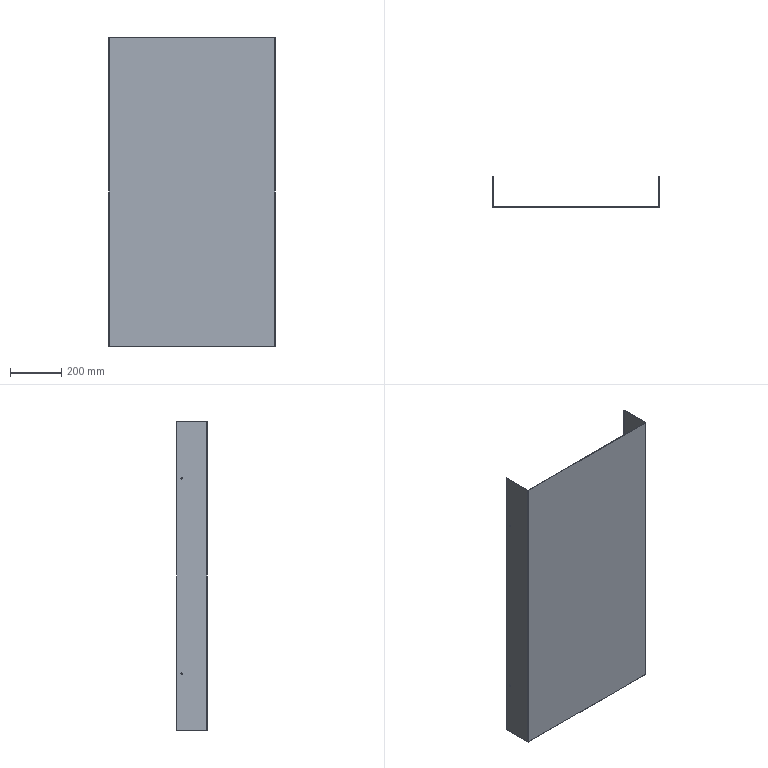Part | SolidWorks | features FlatPattern 1, ICE 1, SMBaseFlange 1, SheetMetal 1 | 1 solid | 30 faces | box 648 x 120 x 1198 mm | volume 2114266 mm3 | plane 18 | cylinder 12 | commonest cylinder face diameters 6 x8 1.473 x2 5.473 x2
STEP:
#1=CARTESIAN_POINT('',(2.,100.,-383.));
#2=VERTEX_POINT('',#1);
#3=CARTESIAN_POINT('',(2.,100.,-377.));
#4=VERTEX_POINT('',#3);
#5=CARTESIAN_POINT('',(2.,100.,-380.));
#6=DIRECTION('',(-1.,0.,0.));
#7=DIRECTION('',(0.,0.,1.));
#8=AXIS2_PLACEMENT_3D('',#5,#6,#7);
#9=CIRCLE('',#8,3.);
#10=EDGE_CURVE('',#2,#4,#9,.T.);
#11=ORIENTED_EDGE('',*,*,#10,.F.);
#12=CARTESIAN_POINT('',(0.,100.,-383.));
#13=VERTEX_POINT('',#12);
#14=CARTESIAN_POINT('',(648.,100.,-383.));
#15=DIRECTION('',(-1.,0.,0.));
#16=VECTOR('',#15,1000.);
#17=LINE('',#14,#16);
#18=EDGE_CURVE('',#2,#13,#17,.T.);
#19=ORIENTED_EDGE('',*,*,#18,.T.);
#20=CARTESIAN_POINT('',(0.,100.,-377.));
#21=VERTEX_POINT('',#20);
#22=CARTESIAN_POINT('',(0.,100.,-380.));
#23=DIRECTION('',(-1.,0.,0.));
#24=DIRECTION('',(0.,0.,1.));
#25=AXIS2_PLACEMENT_3D('',#22,#23,#24);
#26=CIRCLE('',#25,3.);
#27=EDGE_CURVE('',#13,#21,#26,.T.);
#28=ORIENTED_EDGE('',*,*,#27,.T.);
#29=CARTESIAN_POINT('',(648.,100.,-377.));
#30=DIRECTION('',(-1.,0.,0.));
#31=VECTOR('',#30,1000.);
#32=LINE('',#29,#31);
#33=EDGE_CURVE('',#4,#21,#32,.T.);
#34=ORIENTED_EDGE('',*,*,#33,.F.);
#35=EDGE_LOOP('',(#11,#19,#28,#34));
#36=FACE_OUTER_BOUND('',#35,.T.);
#37=CARTESIAN_POINT('',(648.,100.,-380.));
#38=DIRECTION('',(-1.,0.,0.));
#39=DIRECTION('',(0.,0.,1.));
#40=AXIS2_PLACEMENT_3D('',#37,#38,#39);
#41=CYLINDRICAL_SURFACE('',#40,3.);
#42=ADVANCED_FACE('',(#36),#41,.F.);
#43=CARTESIAN_POINT('',(2.,100.,377.));
#44=VERTEX_POINT('',#43);
#45=CARTESIAN_POINT('',(2.,100.,383.));
#46=VERTEX_POINT('',#45);
#47=CARTESIAN_POINT('',(2.,100.,380.));
#48=DIRECTION('',(-1.,0.,0.));
#49=DIRECTION('',(0.,0.,1.));
#50=AXIS2_PLACEMENT_3D('',#47,#48,#49);
#51=CIRCLE('',#50,3.);
#52=EDGE_CURVE('',#44,#46,#51,.T.);
#53=ORIENTED_EDGE('',*,*,#52,.F.);
#54=CARTESIAN_POINT('',(0.,100.,377.));
#55=VERTEX_POINT('',#54);
#56=CARTESIAN_POINT('',(648.,100.,377.));
#57=DIRECTION('',(-1.,0.,0.));
#58=VECTOR('',#57,1000.);
#59=LINE('',#56,#58);
#60=EDGE_CURVE('',#44,#55,#59,.T.);
#61=ORIENTED_EDGE('',*,*,#60,.T.);
#62=CARTESIAN_POINT('',(0.,100.,383.));
#63=VERTEX_POINT('',#62);
#64=CARTESIAN_POINT('',(0.,100.,380.));
#65=DIRECTION('',(-1.,0.,0.));
#66=DIRECTION('',(0.,0.,1.));
#67=AXIS2_PLACEMENT_3D('',#64,#65,#66);
#68=CIRCLE('',#67,3.);
#69=EDGE_CURVE('',#55,#63,#68,.T.);
#70=ORIENTED_EDGE('',*,*,#69,.T.);
#71=CARTESIAN_POINT('',(648.,100.,383.));
#72=DIRECTION('',(-1.,0.,0.));
#73=VECTOR('',#72,1000.);
#74=LINE('',#71,#73);
#75=EDGE_CURVE('',#46,#63,#74,.T.);
#76=ORIENTED_EDGE('',*,*,#75,.F.);
#77=EDGE_LOOP('',(#53,#61,#70,#76));
#78=FACE_OUTER_BOUND('',#77,.T.);
#79=CARTESIAN_POINT('',(648.,100.,380.));
#80=DIRECTION('',(-1.,0.,0.));
#81=DIRECTION('',(0.,0.,1.));
#82=AXIS2_PLACEMENT_3D('',#79,#80,#81);
#83=CYLINDRICAL_SURFACE('',#82,3.);
#84=ADVANCED_FACE('',(#78),#83,.F.);
#85=CARTESIAN_POINT('',(648.,100.,-383.));
#86=VERTEX_POINT('',#85);
#87=CARTESIAN_POINT('',(648.,100.,-377.));
#88=VERTEX_POINT('',#87);
#89=CARTESIAN_POINT('',(648.,100.,-380.));
#90=DIRECTION('',(-1.,0.,0.));
#91=DIRECTION('',(0.,0.,1.));
#92=AXIS2_PLACEMENT_3D('',#89,#90,#91);
#93=CIRCLE('',#92,3.);
#94=EDGE_CURVE('',#86,#88,#93,.T.);
#95=ORIENTED_EDGE('',*,*,#94,.F.);
#96=CARTESIAN_POINT('',(646.,100.,-383.));
#97=VERTEX_POINT('',#96);
#98=CARTESIAN_POINT('',(648.,100.,-383.));
#99=DIRECTION('',(-1.,0.,0.));
#100=VECTOR('',#99,1000.);
#101=LINE('',#98,#100);
#102=EDGE_CURVE('',#86,#97,#101,.T.);
#103=ORIENTED_EDGE('',*,*,#102,.T.);
#104=CARTESIAN_POINT('',(646.,100.,-377.));
#105=VERTEX_POINT('',#104);
#106=CARTESIAN_POINT('',(646.,100.,-380.));
#107=DIRECTION('',(1.,0.,0.));
#108=DIRECTION('',(0.,0.,-1.));
#109=AXIS2_PLACEMENT_3D('',#106,#107,#108);
#110=CIRCLE('',#109,3.);
#111=EDGE_CURVE('',#105,#97,#110,.T.);
#112=ORIENTED_EDGE('',*,*,#111,.F.);
#113=CARTESIAN_POINT('',(648.,100.,-377.));
#114=DIRECTION('',(-1.,0.,0.));
#115=VECTOR('',#114,1000.);
#116=LINE('',#113,#115);
#117=EDGE_CURVE('',#88,#105,#116,.T.);
#118=ORIENTED_EDGE('',*,*,#117,.F.);
#119=EDGE_LOOP('',(#95,#103,#112,#118));
#120=FACE_OUTER_BOUND('',#119,.T.);
#121=CARTESIAN_POINT('',(648.,100.,-380.));
#122=DIRECTION('',(-1.,0.,0.));
#123=DIRECTION('',(0.,0.,1.));
#124=AXIS2_PLACEMENT_3D('',#121,#122,#123);
#125=CYLINDRICAL_SURFACE('',#124,3.);
#126=ADVANCED_FACE('',(#120),#125,.F.);
#127=CARTESIAN_POINT('',(648.,100.,377.));
#128=VERTEX_POINT('',#127);
#129=CARTESIAN_POINT('',(648.,100.,383.));
#130=VERTEX_POINT('',#129);
#131=CARTESIAN_POINT('',(648.,100.,380.));
#132=DIRECTION('',(-1.,0.,0.));
#133=DIRECTION('',(0.,0.,1.));
#134=AXIS2_PLACEMENT_3D('',#131,#132,#133);
#135=CIRCLE('',#134,3.);
#136=EDGE_CURVE('',#128,#130,#135,.T.);
#137=ORIENTED_EDGE('',*,*,#136,.F.);
#138=CARTESIAN_POINT('',(646.,100.,377.));
#139=VERTEX_POINT('',#138);
#140=CARTESIAN_POINT('',(648.,100.,377.));
#141=DIRECTION('',(-1.,0.,0.));
#142=VECTOR('',#141,1000.);
#143=LINE('',#140,#142);
#144=EDGE_CURVE('',#128,#139,#143,.T.);
#145=ORIENTED_EDGE('',*,*,#144,.T.);
#146=CARTESIAN_POINT('',(646.,100.,383.));
#147=VERTEX_POINT('',#146);
#148=CARTESIAN_POINT('',(646.,100.,380.));
#149=DIRECTION('',(1.,0.,0.));
#150=DIRECTION('',(0.,0.,-1.));
#151=AXIS2_PLACEMENT_3D('',#148,#149,#150);
#152=CIRCLE('',#151,3.);
#153=EDGE_CURVE('',#147,#139,#152,.T.);
#154=ORIENTED_EDGE('',*,*,#153,.F.);
#155=CARTESIAN_POINT('',(648.,100.,383.));
#156=DIRECTION('',(-1.,0.,0.));
#157=VECTOR('',#156,1000.);
#158=LINE('',#155,#157);
#159=EDGE_CURVE('',#130,#147,#158,.T.);
#160=ORIENTED_EDGE('',*,*,#159,.F.);
#161=EDGE_LOOP('',(#137,#145,#154,#160));
#162=FACE_OUTER_BOUND('',#161,.T.);
#163=CARTESIAN_POINT('',(648.,100.,380.));
#164=DIRECTION('',(-1.,0.,0.));
#165=DIRECTION('',(0.,0.,1.));
#166=AXIS2_PLACEMENT_3D('',#163,#164,#165);
#167=CYLINDRICAL_SURFACE('',#166,3.);
#168=ADVANCED_FACE('',(#162),#167,.F.);
#169=CARTESIAN_POINT('',(645.263,0.,599.));
#170=VERTEX_POINT('',#169);
#171=CARTESIAN_POINT('',(645.263,2.,599.));
#172=VERTEX_POINT('',#171);
#173=CARTESIAN_POINT('',(645.263,0.,599.));
#174=DIRECTION('',(0.,1.,0.));
#175=VECTOR('',#174,1000.);
#176=LINE('',#173,#175);
#177=EDGE_CURVE('',#170,#172,#176,.T.);
#178=ORIENTED_EDGE('',*,*,#177,.F.);
#179=CARTESIAN_POINT('',(648.,2.737,599.));
#180=VERTEX_POINT('',#179);
#181=CARTESIAN_POINT('',(645.263,2.737,599.));
#182=DIRECTION('',(0.,0.,-1.));
#183=DIRECTION('',(1.,0.,0.));
#184=AXIS2_PLACEMENT_3D('',#181,#182,#183);
#185=CIRCLE('',#184,2.737);
#186=EDGE_CURVE('',#180,#170,#185,.T.);
#187=ORIENTED_EDGE('',*,*,#186,.F.);
#188=CARTESIAN_POINT('',(646.,2.737,599.));
#189=VERTEX_POINT('',#188);
#190=CARTESIAN_POINT('',(646.,2.737,599.));
#191=DIRECTION('',(1.,0.,0.));
#192=VECTOR('',#191,1000.);
#193=LINE('',#190,#192);
#194=EDGE_CURVE('',#189,#180,#193,.T.);
#195=ORIENTED_EDGE('',*,*,#194,.F.);
#196=CARTESIAN_POINT('',(645.263,2.737,599.));
#197=DIRECTION('',(0.,0.,-1.));
#198=DIRECTION('',(1.,0.,0.));
#199=AXIS2_PLACEMENT_3D('',#196,#197,#198);
#200=CIRCLE('',#199,0.7366);
#201=EDGE_CURVE('',#189,#172,#200,.T.);
#202=ORIENTED_EDGE('',*,*,#201,.T.);
#203=EDGE_LOOP('',(#178,#187,#195,#202));
#204=FACE_OUTER_BOUND('',#203,.T.);
#205=CARTESIAN_POINT('',(645.263,0.,599.));
#206=DIRECTION('',(0.,0.,1.));
#207=DIRECTION('',(1.,0.,0.));
#208=AXIS2_PLACEMENT_3D('',#205,#206,#207);
#209=PLANE('',#208);
#210=ADVANCED_FACE('',(#204),#209,.T.);
#211=CARTESIAN_POINT('',(2.737,0.,599.));
#212=VERTEX_POINT('',#211);
#213=CARTESIAN_POINT('',(0.,0.,599.));
#214=DIRECTION('',(-1.,0.,0.));
#215=VECTOR('',#214,1000.);
#216=LINE('',#213,#215);
#217=EDGE_CURVE('',#170,#212,#216,.T.);
#218=ORIENTED_EDGE('',*,*,#217,.F.);
#219=ORIENTED_EDGE('',*,*,#177,.T.);
#220=CARTESIAN_POINT('',(2.737,2.,599.));
#221=VERTEX_POINT('',#220);
#222=CARTESIAN_POINT('',(0.,2.,599.));
#223=DIRECTION('',(-1.,0.,0.));
#224=VECTOR('',#223,1000.);
#225=LINE('',#222,#224);
#226=EDGE_CURVE('',#172,#221,#225,.T.);
#227=ORIENTED_EDGE('',*,*,#226,.T.);
#228=CARTESIAN_POINT('',(2.737,2.,599.));
#229=DIRECTION('',(0.,-1.,0.));
#230=VECTOR('',#229,1000.);
#231=LINE('',#228,#230);
#232=EDGE_CURVE('',#221,#212,#231,.T.);
#233=ORIENTED_EDGE('',*,*,#232,.T.);
#234=EDGE_LOOP('',(#218,#219,#227,#233));
#235=FACE_OUTER_BOUND('',#234,.T.);
#236=CARTESIAN_POINT('',(646.,2.737,599.));
#237=DIRECTION('',(0.,0.,1.));
#238=DIRECTION('',(1.,0.,0.));
#239=AXIS2_PLACEMENT_3D('',#236,#237,#238);
#240=PLANE('',#239);
#241=ADVANCED_FACE('',(#235),#240,.T.);
#242=CARTESIAN_POINT('',(648.,2.737,-599.));
#243=VERTEX_POINT('',#242);
#244=CARTESIAN_POINT('',(646.,2.737,-599.));
#245=VERTEX_POINT('',#244);
#246=CARTESIAN_POINT('',(648.,2.737,-599.));
#247=DIRECTION('',(-1.,0.,0.));
#248=VECTOR('',#247,1000.);
#249=LINE('',#246,#248);
#250=EDGE_CURVE('',#243,#245,#249,.T.);
#251=ORIENTED_EDGE('',*,*,#250,.F.);
#252=CARTESIAN_POINT('',(645.263,0.,-599.));
#253=VERTEX_POINT('',#252);
#254=CARTESIAN_POINT('',(645.263,2.737,-599.));
#255=DIRECTION('',(0.,0.,-1.));
#256=DIRECTION('',(1.,0.,0.));
#257=AXIS2_PLACEMENT_3D('',#254,#255,#256);
#258=CIRCLE('',#257,2.737);
#259=EDGE_CURVE('',#243,#253,#258,.T.);
#260=ORIENTED_EDGE('',*,*,#259,.T.);
#261=CARTESIAN_POINT('',(645.263,2.,-599.));
#262=VERTEX_POINT('',#261);
#263=CARTESIAN_POINT('',(645.263,2.,-599.));
#264=DIRECTION('',(0.,-1.,0.));
#265=VECTOR('',#264,1000.);
#266=LINE('',#263,#265);
#267=EDGE_CURVE('',#262,#253,#266,.T.);
#268=ORIENTED_EDGE('',*,*,#267,.F.);
#269=CARTESIAN_POINT('',(645.263,2.737,-599.));
#270=DIRECTION('',(0.,0.,-1.));
#271=DIRECTION('',(1.,0.,0.));
#272=AXIS2_PLACEMENT_3D('',#269,#270,#271);
#273=CIRCLE('',#272,0.7366);
#274=EDGE_CURVE('',#245,#262,#273,.T.);
#275=ORIENTED_EDGE('',*,*,#274,.F.);
#276=EDGE_LOOP('',(#251,#260,#268,#275));
#277=FACE_OUTER_BOUND('',#276,.T.);
#278=CARTESIAN_POINT('',(648.,2.737,-599.));
#279=DIRECTION('',(0.,0.,-1.));
#280=DIRECTION('',(-1.,0.,0.));
#281=AXIS2_PLACEMENT_3D('',#278,#279,#280);
#282=PLANE('',#281);
#283=ADVANCED_FACE('',(#277),#282,.T.);
#284=CARTESIAN_POINT('',(648.,120.,-599.));
#285=VERTEX_POINT('',#284);
#286=CARTESIAN_POINT('',(648.,0.,-599.));
#287=DIRECTION('',(0.,-1.,0.));
#288=VECTOR('',#287,1000.);
#289=LINE('',#286,#288);
#290=EDGE_CURVE('',#285,#243,#289,.T.);
#291=ORIENTED_EDGE('',*,*,#290,.T.);
#292=ORIENTED_EDGE('',*,*,#250,.T.);
#293=CARTESIAN_POINT('',(646.,120.,-599.));
#294=VERTEX_POINT('',#293);
#295=CARTESIAN_POINT('',(646.,0.,-599.));
#296=DIRECTION('',(0.,-1.,0.));
#297=VECTOR('',#296,1000.);
#298=LINE('',#295,#297);
#299=EDGE_CURVE('',#294,#245,#298,.T.);
#300=ORIENTED_EDGE('',*,*,#299,.F.);
#301=CARTESIAN_POINT('',(646.,120.,-599.));
#302=DIRECTION('',(1.,0.,0.));
#303=VECTOR('',#302,1000.);
#304=LINE('',#301,#303);
#305=EDGE_CURVE('',#294,#285,#304,.T.);
#306=ORIENTED_EDGE('',*,*,#305,.T.);
#307=EDGE_LOOP('',(#291,#292,#300,#306));
#308=FACE_OUTER_BOUND('',#307,.T.);
#309=CARTESIAN_POINT('',(645.263,2.,-599.));
#310=DIRECTION('',(0.,0.,-1.));
#311=DIRECTION('',(-1.,0.,0.));
#312=AXIS2_PLACEMENT_3D('',#309,#310,#311);
#313=PLANE('',#312);
#314=ADVANCED_FACE('',(#308),#313,.T.);
#315=CARTESIAN_POINT('',(0.,2.737,599.));
#316=VERTEX_POINT('',#315);
#317=CARTESIAN_POINT('',(2.,2.737,599.));
#318=VERTEX_POINT('',#317);
#319=CARTESIAN_POINT('',(0.,2.737,599.));
#320=DIRECTION('',(1.,0.,0.));
#321=VECTOR('',#320,1000.);
#322=LINE('',#319,#321);
#323=EDGE_CURVE('',#316,#318,#322,.T.);
#324=ORIENTED_EDGE('',*,*,#323,.F.);
#325=CARTESIAN_POINT('',(2.737,2.737,599.));
#326=DIRECTION('',(0.,0.,-1.));
#327=DIRECTION('',(1.,0.,0.));
#328=AXIS2_PLACEMENT_3D('',#325,#326,#327);
#329=CIRCLE('',#328,2.737);
#330=EDGE_CURVE('',#212,#316,#329,.T.);
#331=ORIENTED_EDGE('',*,*,#330,.F.);
#332=ORIENTED_EDGE('',*,*,#232,.F.);
#333=CARTESIAN_POINT('',(2.737,2.737,599.));
#334=DIRECTION('',(0.,0.,-1.));
#335=DIRECTION('',(1.,0.,0.));
#336=AXIS2_PLACEMENT_3D('',#333,#334,#335);
#337=CIRCLE('',#336,0.7366);
#338=EDGE_CURVE('',#221,#318,#337,.T.);
#339=ORIENTED_EDGE('',*,*,#338,.T.);
#340=EDGE_LOOP('',(#324,#331,#332,#339));
#341=FACE_OUTER_BOUND('',#340,.T.);
#342=CARTESIAN_POINT('',(0.,2.737,599.));
#343=DIRECTION('',(0.,0.,1.));
#344=DIRECTION('',(1.,0.,0.));
#345=AXIS2_PLACEMENT_3D('',#342,#343,#344);
#346=PLANE('',#345);
#347=ADVANCED_FACE('',(#341),#346,.T.);
#348=CARTESIAN_POINT('',(0.,120.,599.));
#349=VERTEX_POINT('',#348);
#350=CARTESIAN_POINT('',(0.,0.,599.));
#351=DIRECTION('',(0.,1.,0.));
#352=VECTOR('',#351,1000.);
#353=LINE('',#350,#352);
#354=EDGE_CURVE('',#316,#349,#353,.T.);
#355=ORIENTED_EDGE('',*,*,#354,.F.);
#356=ORIENTED_EDGE('',*,*,#323,.T.);
#357=CARTESIAN_POINT('',(2.,120.,599.));
#358=VERTEX_POINT('',#357);
#359=CARTESIAN_POINT('',(2.,0.,599.));
#360=DIRECTION('',(0.,1.,0.));
#361=VECTOR('',#360,1000.);
#362=LINE('',#359,#361);
#363=EDGE_CURVE('',#318,#358,#362,.T.);
#364=ORIENTED_EDGE('',*,*,#363,.T.);
#365=CARTESIAN_POINT('',(0.,120.,599.));
#366=DIRECTION('',(1.,0.,0.));
#367=VECTOR('',#366,1000.);
#368=LINE('',#365,#367);
#369=EDGE_CURVE('',#349,#358,#368,.T.);
#370=ORIENTED_EDGE('',*,*,#369,.F.);
#371=EDGE_LOOP('',(#355,#356,#364,#370));
#372=FACE_OUTER_BOUND('',#371,.T.);
#373=CARTESIAN_POINT('',(2.737,2.,599.));
#374=DIRECTION('',(0.,0.,1.));
#375=DIRECTION('',(1.,0.,0.));
#376=AXIS2_PLACEMENT_3D('',#373,#374,#375);
#377=PLANE('',#376);
#378=ADVANCED_FACE('',(#372),#377,.T.);
#379=CARTESIAN_POINT('',(2.737,0.,-599.));
#380=VERTEX_POINT('',#379);
#381=CARTESIAN_POINT('',(2.737,2.,-599.));
#382=VERTEX_POINT('',#381);
#383=CARTESIAN_POINT('',(2.737,0.,-599.));
#384=DIRECTION('',(0.,1.,0.));
#385=VECTOR('',#384,1000.);
#386=LINE('',#383,#385);
#387=EDGE_CURVE('',#380,#382,#386,.T.);
#388=ORIENTED_EDGE('',*,*,#387,.F.);
#389=CARTESIAN_POINT('',(0.,2.737,-599.));
#390=VERTEX_POINT('',#389);
#391=CARTESIAN_POINT('',(2.737,2.737,-599.));
#392=DIRECTION('',(0.,0.,-1.));
#393=DIRECTION('',(1.,0.,0.));
#394=AXIS2_PLACEMENT_3D('',#391,#392,#393);
#395=CIRCLE('',#394,2.737);
#396=EDGE_CURVE('',#380,#390,#395,.T.);
#397=ORIENTED_EDGE('',*,*,#396,.T.);
#398=CARTESIAN_POINT('',(2.,2.737,-599.));
#399=VERTEX_POINT('',#398);
#400=CARTESIAN_POINT('',(2.,2.737,-599.));
#401=DIRECTION('',(-1.,0.,0.));
#402=VECTOR('',#401,1000.);
#403=LINE('',#400,#402);
#404=EDGE_CURVE('',#399,#390,#403,.T.);
#405=ORIENTED_EDGE('',*,*,#404,.F.);
#406=CARTESIAN_POINT('',(2.737,2.737,-599.));
#407=DIRECTION('',(0.,0.,-1.));
#408=DIRECTION('',(1.,0.,0.));
#409=AXIS2_PLACEMENT_3D('',#406,#407,#408);
#410=CIRCLE('',#409,0.7366);
#411=EDGE_CURVE('',#382,#399,#410,.T.);
#412=ORIENTED_EDGE('',*,*,#411,.F.);
#413=EDGE_LOOP('',(#388,#397,#405,#412));
#414=FACE_OUTER_BOUND('',#413,.T.);
#415=CARTESIAN_POINT('',(2.737,0.,-599.));
#416=DIRECTION('',(0.,0.,-1.));
#417=DIRECTION('',(-1.,0.,0.));
#418=AXIS2_PLACEMENT_3D('',#415,#416,#417);
#419=PLANE('',#418);
#420=ADVANCED_FACE('',(#414),#419,.T.);
#421=CARTESIAN_POINT('',(0.,0.,-599.));
#422=DIRECTION('',(-1.,0.,0.));
#423=VECTOR('',#422,1000.);
#424=LINE('',#421,#423);
#425=EDGE_CURVE('',#253,#380,#424,.T.);
#426=ORIENTED_EDGE('',*,*,#425,.T.);
#427=ORIENTED_EDGE('',*,*,#387,.T.);
#428=CARTESIAN_POINT('',(0.,2.,-599.));
#429=DIRECTION('',(-1.,0.,0.));
#430=VECTOR('',#429,1000.);
#431=LINE('',#428,#430);
#432=EDGE_CURVE('',#262,#382,#431,.T.);
#433=ORIENTED_EDGE('',*,*,#432,.F.);
#434=ORIENTED_EDGE('',*,*,#267,.T.);
#435=EDGE_LOOP('',(#426,#427,#433,#434));
#436=FACE_OUTER_BOUND('',#435,.T.);
#437=CARTESIAN_POINT('',(2.,2.737,-599.));
#438=DIRECTION('',(0.,0.,-1.));
#439=DIRECTION('',(-1.,0.,0.));
#440=AXIS2_PLACEMENT_3D('',#437,#438,#439);
#441=PLANE('',#440);
#442=ADVANCED_FACE('',(#436),#441,.T.);
#443=CARTESIAN_POINT('',(2.,100.,-380.));
#444=DIRECTION('',(-1.,0.,0.));
#445=DIRECTION('',(0.,0.,1.));
#446=AXIS2_PLACEMENT_3D('',#443,#444,#445);
#447=CIRCLE('',#446,3.);
#448=EDGE_CURVE('',#4,#2,#447,.T.);
#449=ORIENTED_EDGE('',*,*,#448,.T.);
#450=ORIENTED_EDGE('',*,*,#10,.T.);
#451=EDGE_LOOP('',(#449,#450));
#452=FACE_BOUND('',#451,.T.);
#453=CARTESIAN_POINT('',(2.,100.,380.));
#454=DIRECTION('',(-1.,0.,0.));
#455=DIRECTION('',(0.,0.,1.));
#456=AXIS2_PLACEMENT_3D('',#453,#454,#455);
#457=CIRCLE('',#456,3.);
#458=EDGE_CURVE('',#46,#44,#457,.T.);
#459=ORIENTED_EDGE('',*,*,#458,.T.);
#460=ORIENTED_EDGE('',*,*,#52,.T.);
#461=EDGE_LOOP('',(#459,#460));
#462=FACE_BOUND('',#461,.T.);
#463=CARTESIAN_POINT('',(2.,120.,-599.));
#464=VERTEX_POINT('',#463);
#465=CARTESIAN_POINT('',(2.,0.,-599.));
#466=DIRECTION('',(0.,1.,0.));
#467=VECTOR('',#466,1000.);
#468=LINE('',#465,#467);
#469=EDGE_CURVE('',#399,#464,#468,.T.);
#470=ORIENTED_EDGE('',*,*,#469,.T.);
#471=CARTESIAN_POINT('',(2.,120.,599.));
#472=DIRECTION('',(0.,0.,-1.));
#473=VECTOR('',#472,1000.);
#474=LINE('',#471,#473);
#475=EDGE_CURVE('',#358,#464,#474,.T.);
#476=ORIENTED_EDGE('',*,*,#475,.F.);
#477=ORIENTED_EDGE('',*,*,#363,.F.);
#478=CARTESIAN_POINT('',(2.,2.737,599.));
#479=DIRECTION('',(0.,0.,-1.));
#480=VECTOR('',#479,1000.);
#481=LINE('',#478,#480);
#482=EDGE_CURVE('',#318,#399,#481,.T.);
#483=ORIENTED_EDGE('',*,*,#482,.T.);
#484=EDGE_LOOP('',(#470,#476,#477,#483));
#485=FACE_OUTER_BOUND('',#484,.T.);
#486=CARTESIAN_POINT('',(2.,0.,599.));
#487=DIRECTION('',(-1.,0.,0.));
#488=DIRECTION('',(0.,0.,1.));
#489=AXIS2_PLACEMENT_3D('',#486,#487,#488);
#490=PLANE('',#489);
#491=ADVANCED_FACE('',(#452,#462,#485),#490,.F.);
#492=CARTESIAN_POINT('',(0.,120.,-599.));
#493=VERTEX_POINT('',#492);
#494=CARTESIAN_POINT('',(0.,120.,-599.));
#495=DIRECTION('',(1.,0.,0.));
#496=VECTOR('',#495,1000.);
#497=LINE('',#494,#496);
#498=EDGE_CURVE('',#493,#464,#497,.T.);
#499=ORIENTED_EDGE('',*,*,#498,.F.);
#500=CARTESIAN_POINT('',(0.,120.,599.));
#501=DIRECTION('',(0.,0.,-1.));
#502=VECTOR('',#501,1000.);
#503=LINE('',#500,#502);
#504=EDGE_CURVE('',#349,#493,#503,.T.);
#505=ORIENTED_EDGE('',*,*,#504,.F.);
#506=ORIENTED_EDGE('',*,*,#369,.T.);
#507=ORIENTED_EDGE('',*,*,#475,.T.);
#508=EDGE_LOOP('',(#499,#505,#506,#507));
#509=FACE_OUTER_BOUND('',#508,.T.);
#510=CARTESIAN_POINT('',(0.,120.,599.));
#511=DIRECTION('',(0.,1.,0.));
#512=DIRECTION('',(0.,0.,1.));
#513=AXIS2_PLACEMENT_3D('',#510,#511,#512);
#514=PLANE('',#513);
#515=ADVANCED_FACE('',(#509),#514,.T.);
#516=CARTESIAN_POINT('',(0.,100.,-380.));
#517=DIRECTION('',(-1.,0.,0.));
#518=DIRECTION('',(0.,0.,1.));
#519=AXIS2_PLACEMENT_3D('',#516,#517,#518);
#520=CIRCLE('',#519,3.);
#521=EDGE_CURVE('',#21,#13,#520,.T.);
#522=ORIENTED_EDGE('',*,*,#521,.F.);
#523=ORIENTED_EDGE('',*,*,#27,.F.);
#524=EDGE_LOOP('',(#522,#523));
#525=FACE_BOUND('',#524,.T.);
#526=CARTESIAN_POINT('',(0.,100.,380.));
#527=DIRECTION('',(-1.,0.,0.));
#528=DIRECTION('',(0.,0.,1.));
#529=AXIS2_PLACEMENT_3D('',#526,#527,#528);
#530=CIRCLE('',#529,3.);
#531=EDGE_CURVE('',#63,#55,#530,.T.);
#532=ORIENTED_EDGE('',*,*,#531,.F.);
#533=ORIENTED_EDGE('',*,*,#69,.F.);
#534=EDGE_LOOP('',(#532,#533));
#535=FACE_BOUND('',#534,.T.);
#536=CARTESIAN_POINT('',(0.,0.,-599.));
#537=DIRECTION('',(0.,1.,0.));
#538=VECTOR('',#537,1000.);
#539=LINE('',#536,#538);
#540=EDGE_CURVE('',#390,#493,#539,.T.);
#541=ORIENTED_EDGE('',*,*,#540,.F.);
#542=CARTESIAN_POINT('',(0.,2.737,599.));
#543=DIRECTION('',(0.,0.,-1.));
#544=VECTOR('',#543,1000.);
#545=LINE('',#542,#544);
#546=EDGE_CURVE('',#316,#390,#545,.T.);
#547=ORIENTED_EDGE('',*,*,#546,.F.);
#548=ORIENTED_EDGE('',*,*,#354,.T.);
#549=ORIENTED_EDGE('',*,*,#504,.T.);
#550=EDGE_LOOP('',(#541,#547,#548,#549));
#551=FACE_OUTER_BOUND('',#550,.T.);
#552=CARTESIAN_POINT('',(0.,0.,599.));
#553=DIRECTION('',(-1.,0.,0.));
#554=DIRECTION('',(0.,0.,1.));
#555=AXIS2_PLACEMENT_3D('',#552,#553,#554);
#556=PLANE('',#555);
#557=ADVANCED_FACE('',(#525,#535,#551),#556,.T.);
#558=ORIENTED_EDGE('',*,*,#396,.F.);
#559=CARTESIAN_POINT('',(2.737,0.,599.));
#560=DIRECTION('',(0.,0.,-1.));
#561=VECTOR('',#560,1000.);
#562=LINE('',#559,#561);
#563=EDGE_CURVE('',#212,#380,#562,.T.);
#564=ORIENTED_EDGE('',*,*,#563,.F.);
#565=ORIENTED_EDGE('',*,*,#330,.T.);
#566=ORIENTED_EDGE('',*,*,#546,.T.);
#567=EDGE_LOOP('',(#558,#564,#565,#566));
#568=FACE_OUTER_BOUND('',#567,.T.);
#569=CARTESIAN_POINT('',(2.737,2.737,599.));
#570=DIRECTION('',(0.,0.,-1.));
#571=DIRECTION('',(-1.,0.,0.));
#572=AXIS2_PLACEMENT_3D('',#569,#570,#571);
#573=CYLINDRICAL_SURFACE('',#572,2.737);
#574=ADVANCED_FACE('',(#568),#573,.T.);
#575=ORIENTED_EDGE('',*,*,#425,.F.);
#576=CARTESIAN_POINT('',(645.263,0.,599.));
#577=DIRECTION('',(0.,0.,-1.));
#578=VECTOR('',#577,1000.);
#579=LINE('',#576,#578);
#580=EDGE_CURVE('',#170,#253,#579,.T.);
#581=ORIENTED_EDGE('',*,*,#580,.F.);
#582=ORIENTED_EDGE('',*,*,#217,.T.);
#583=ORIENTED_EDGE('',*,*,#563,.T.);
#584=EDGE_LOOP('',(#575,#581,#582,#583));
#585=FACE_OUTER_BOUND('',#584,.T.);
#586=CARTESIAN_POINT('',(0.,0.,599.));
#587=DIRECTION('',(0.,-1.,0.));
#588=DIRECTION('',(0.,0.,-1.));
#589=AXIS2_PLACEMENT_3D('',#586,#587,#588);
#590=PLANE('',#589);
#591=ADVANCED_FACE('',(#585),#590,.T.);
#592=ORIENTED_EDGE('',*,*,#259,.F.);
#593=CARTESIAN_POINT('',(648.,2.737,599.));
#594=DIRECTION('',(0.,0.,-1.));
#595=VECTOR('',#594,1000.);
#596=LINE('',#593,#595);
#597=EDGE_CURVE('',#180,#243,#596,.T.);
#598=ORIENTED_EDGE('',*,*,#597,.F.);
#599=ORIENTED_EDGE('',*,*,#186,.T.);
#600=ORIENTED_EDGE('',*,*,#580,.T.);
#601=EDGE_LOOP('',(#592,#598,#599,#600));
#602=FACE_OUTER_BOUND('',#601,.T.);
#603=CARTESIAN_POINT('',(645.263,2.737,599.));
#604=DIRECTION('',(0.,0.,-1.));
#605=DIRECTION('',(-1.,0.,0.));
#606=AXIS2_PLACEMENT_3D('',#603,#604,#605);
#607=CYLINDRICAL_SURFACE('',#606,2.737);
#608=ADVANCED_FACE('',(#602),#607,.T.);
#609=CARTESIAN_POINT('',(648.,100.,-380.));
#610=DIRECTION('',(-1.,0.,0.));
#611=DIRECTION('',(0.,0.,1.));
#612=AXIS2_PLACEMENT_3D('',#609,#610,#611);
#613=CIRCLE('',#612,3.);
#614=EDGE_CURVE('',#88,#86,#613,.T.);
#615=ORIENTED_EDGE('',*,*,#614,.T.);
#616=ORIENTED_EDGE('',*,*,#94,.T.);
#617=EDGE_LOOP('',(#615,#616));
#618=FACE_BOUND('',#617,.T.);
#619=CARTESIAN_POINT('',(648.,100.,380.));
#620=DIRECTION('',(-1.,0.,0.));
#621=DIRECTION('',(0.,0.,1.));
#622=AXIS2_PLACEMENT_3D('',#619,#620,#621);
#623=CIRCLE('',#622,3.);
#624=EDGE_CURVE('',#130,#128,#623,.T.);
#625=ORIENTED_EDGE('',*,*,#624,.T.);
#626=ORIENTED_EDGE('',*,*,#136,.T.);
#627=EDGE_LOOP('',(#625,#626));
#628=FACE_BOUND('',#627,.T.);
#629=ORIENTED_EDGE('',*,*,#290,.F.);
#630=CARTESIAN_POINT('',(648.,120.,599.));
#631=VERTEX_POINT('',#630);
#632=CARTESIAN_POINT('',(648.,120.,599.));
#633=DIRECTION('',(0.,0.,-1.));
#634=VECTOR('',#633,1000.);
#635=LINE('',#632,#634);
#636=EDGE_CURVE('',#631,#285,#635,.T.);
#637=ORIENTED_EDGE('',*,*,#636,.F.);
#638=CARTESIAN_POINT('',(648.,0.,599.));
#639=DIRECTION('',(0.,-1.,0.));
#640=VECTOR('',#639,1000.);
#641=LINE('',#638,#640);
#642=EDGE_CURVE('',#631,#180,#641,.T.);
#643=ORIENTED_EDGE('',*,*,#642,.T.);
#644=ORIENTED_EDGE('',*,*,#597,.T.);
#645=EDGE_LOOP('',(#629,#637,#643,#644));
#646=FACE_OUTER_BOUND('',#645,.T.);
#647=CARTESIAN_POINT('',(648.,0.,599.));
#648=DIRECTION('',(1.,0.,0.));
#649=DIRECTION('',(0.,0.,-1.));
#650=AXIS2_PLACEMENT_3D('',#647,#648,#649);
#651=PLANE('',#650);
#652=ADVANCED_FACE('',(#618,#628,#646),#651,.T.);
#653=ORIENTED_EDGE('',*,*,#305,.F.);
#654=CARTESIAN_POINT('',(646.,120.,599.));
#655=VERTEX_POINT('',#654);
#656=CARTESIAN_POINT('',(646.,120.,599.));
#657=DIRECTION('',(0.,0.,-1.));
#658=VECTOR('',#657,1000.);
#659=LINE('',#656,#658);
#660=EDGE_CURVE('',#655,#294,#659,.T.);
#661=ORIENTED_EDGE('',*,*,#660,.F.);
#662=CARTESIAN_POINT('',(646.,120.,599.));
#663=DIRECTION('',(1.,0.,0.));
#664=VECTOR('',#663,1000.);
#665=LINE('',#662,#664);
#666=EDGE_CURVE('',#655,#631,#665,.T.);
#667=ORIENTED_EDGE('',*,*,#666,.T.);
#668=ORIENTED_EDGE('',*,*,#636,.T.);
#669=EDGE_LOOP('',(#653,#661,#667,#668));
#670=FACE_OUTER_BOUND('',#669,.T.);
#671=CARTESIAN_POINT('',(646.,120.,599.));
#672=DIRECTION('',(0.,1.,0.));
#673=DIRECTION('',(0.,0.,1.));
#674=AXIS2_PLACEMENT_3D('',#671,#672,#673);
#675=PLANE('',#674);
#676=ADVANCED_FACE('',(#670),#675,.T.);
#677=ORIENTED_EDGE('',*,*,#111,.T.);
#678=CARTESIAN_POINT('',(646.,100.,-380.));
#679=DIRECTION('',(1.,0.,0.));
#680=DIRECTION('',(0.,0.,-1.));
#681=AXIS2_PLACEMENT_3D('',#678,#679,#680);
#682=CIRCLE('',#681,3.);
#683=EDGE_CURVE('',#97,#105,#682,.T.);
#684=ORIENTED_EDGE('',*,*,#683,.T.);
#685=EDGE_LOOP('',(#677,#684));
#686=FACE_BOUND('',#685,.T.);
#687=ORIENTED_EDGE('',*,*,#153,.T.);
#688=CARTESIAN_POINT('',(646.,100.,380.));
#689=DIRECTION('',(1.,0.,0.));
#690=DIRECTION('',(0.,0.,-1.));
#691=AXIS2_PLACEMENT_3D('',#688,#689,#690);
#692=CIRCLE('',#691,3.);
#693=EDGE_CURVE('',#139,#147,#692,.T.);
#694=ORIENTED_EDGE('',*,*,#693,.T.);
#695=EDGE_LOOP('',(#687,#694));
#696=FACE_BOUND('',#695,.T.);
#697=ORIENTED_EDGE('',*,*,#299,.T.);
#698=CARTESIAN_POINT('',(646.,2.737,599.));
#699=DIRECTION('',(0.,0.,-1.));
#700=VECTOR('',#699,1000.);
#701=LINE('',#698,#700);
#702=EDGE_CURVE('',#189,#245,#701,.T.);
#703=ORIENTED_EDGE('',*,*,#702,.F.);
#704=CARTESIAN_POINT('',(646.,0.,599.));
#705=DIRECTION('',(0.,-1.,0.));
#706=VECTOR('',#705,1000.);
#707=LINE('',#704,#706);
#708=EDGE_CURVE('',#655,#189,#707,.T.);
#709=ORIENTED_EDGE('',*,*,#708,.F.);
#710=ORIENTED_EDGE('',*,*,#660,.T.);
#711=EDGE_LOOP('',(#697,#703,#709,#710));
#712=FACE_OUTER_BOUND('',#711,.T.);
#713=CARTESIAN_POINT('',(646.,0.,599.));
#714=DIRECTION('',(1.,0.,0.));
#715=DIRECTION('',(0.,0.,-1.));
#716=AXIS2_PLACEMENT_3D('',#713,#714,#715);
#717=PLANE('',#716);
#718=ADVANCED_FACE('',(#686,#696,#712),#717,.F.);
#719=ORIENTED_EDGE('',*,*,#274,.T.);
#720=CARTESIAN_POINT('',(645.263,2.,599.));
#721=DIRECTION('',(0.,0.,-1.));
#722=VECTOR('',#721,1000.);
#723=LINE('',#720,#722);
#724=EDGE_CURVE('',#172,#262,#723,.T.);
#725=ORIENTED_EDGE('',*,*,#724,.F.);
#726=ORIENTED_EDGE('',*,*,#201,.F.);
#727=ORIENTED_EDGE('',*,*,#702,.T.);
#728=EDGE_LOOP('',(#719,#725,#726,#727));
#729=FACE_OUTER_BOUND('',#728,.T.);
#730=CARTESIAN_POINT('',(645.263,2.737,599.));
#731=DIRECTION('',(0.,0.,-1.));
#732=DIRECTION('',(-1.,0.,0.));
#733=AXIS2_PLACEMENT_3D('',#730,#731,#732);
#734=CYLINDRICAL_SURFACE('',#733,0.7366);
#735=ADVANCED_FACE('',(#729),#734,.F.);
#736=ORIENTED_EDGE('',*,*,#432,.T.);
#737=CARTESIAN_POINT('',(2.737,2.,599.));
#738=DIRECTION('',(0.,0.,-1.));
#739=VECTOR('',#738,1000.);
#740=LINE('',#737,#739);
#741=EDGE_CURVE('',#221,#382,#740,.T.);
#742=ORIENTED_EDGE('',*,*,#741,.F.);
#743=ORIENTED_EDGE('',*,*,#226,.F.);
#744=ORIENTED_EDGE('',*,*,#724,.T.);
#745=EDGE_LOOP('',(#736,#742,#743,#744));
#746=FACE_OUTER_BOUND('',#745,.T.);
#747=CARTESIAN_POINT('',(0.,2.,599.));
#748=DIRECTION('',(0.,-1.,0.));
#749=DIRECTION('',(0.,0.,-1.));
#750=AXIS2_PLACEMENT_3D('',#747,#748,#749);
#751=PLANE('',#750);
#752=ADVANCED_FACE('',(#746),#751,.F.);
#753=ORIENTED_EDGE('',*,*,#411,.T.);
#754=ORIENTED_EDGE('',*,*,#482,.F.);
#755=ORIENTED_EDGE('',*,*,#338,.F.);
#756=ORIENTED_EDGE('',*,*,#741,.T.);
#757=EDGE_LOOP('',(#753,#754,#755,#756));
#758=FACE_OUTER_BOUND('',#757,.T.);
#759=CARTESIAN_POINT('',(2.737,2.737,599.));
#760=DIRECTION('',(0.,0.,-1.));
#761=DIRECTION('',(-1.,0.,0.));
#762=AXIS2_PLACEMENT_3D('',#759,#760,#761);
#763=CYLINDRICAL_SURFACE('',#762,0.7366);
#764=ADVANCED_FACE('',(#758),#763,.F.);
#765=ORIENTED_EDGE('',*,*,#708,.T.);
#766=ORIENTED_EDGE('',*,*,#194,.T.);
#767=ORIENTED_EDGE('',*,*,#642,.F.);
#768=ORIENTED_EDGE('',*,*,#666,.F.);
#769=EDGE_LOOP('',(#765,#766,#767,#768));
#770=FACE_OUTER_BOUND('',#769,.T.);
#771=CARTESIAN_POINT('',(2.737,2.737,599.));
#772=DIRECTION('',(0.,0.,1.));
#773=DIRECTION('',(1.,0.,0.));
#774=AXIS2_PLACEMENT_3D('',#771,#772,#773);
#775=PLANE('',#774);
#776=ADVANCED_FACE('',(#770),#775,.T.);
#777=ORIENTED_EDGE('',*,*,#469,.F.);
#778=ORIENTED_EDGE('',*,*,#404,.T.);
#779=ORIENTED_EDGE('',*,*,#540,.T.);
#780=ORIENTED_EDGE('',*,*,#498,.T.);
#781=EDGE_LOOP('',(#777,#778,#779,#780));
#782=FACE_OUTER_BOUND('',#781,.T.);
#783=CARTESIAN_POINT('',(2.737,2.737,-599.));
#784=DIRECTION('',(0.,0.,1.));
#785=DIRECTION('',(1.,0.,0.));
#786=AXIS2_PLACEMENT_3D('',#783,#784,#785);
#787=PLANE('',#786);
#788=ADVANCED_FACE('',(#782),#787,.F.);
#789=ORIENTED_EDGE('',*,*,#144,.F.);
#790=ORIENTED_EDGE('',*,*,#624,.F.);
#791=ORIENTED_EDGE('',*,*,#159,.T.);
#792=ORIENTED_EDGE('',*,*,#693,.F.);
#793=EDGE_LOOP('',(#789,#790,#791,#792));
#794=FACE_OUTER_BOUND('',#793,.T.);
#795=CARTESIAN_POINT('',(648.,100.,380.));
#796=DIRECTION('',(-1.,0.,0.));
#797=DIRECTION('',(0.,0.,1.));
#798=AXIS2_PLACEMENT_3D('',#795,#796,#797);
#799=CYLINDRICAL_SURFACE('',#798,3.);
#800=ADVANCED_FACE('',(#794),#799,.F.);
#801=ORIENTED_EDGE('',*,*,#102,.F.);
#802=ORIENTED_EDGE('',*,*,#614,.F.);
#803=ORIENTED_EDGE('',*,*,#117,.T.);
#804=ORIENTED_EDGE('',*,*,#683,.F.);
#805=EDGE_LOOP('',(#801,#802,#803,#804));
#806=FACE_OUTER_BOUND('',#805,.T.);
#807=CARTESIAN_POINT('',(648.,100.,-380.));
#808=DIRECTION('',(-1.,0.,0.));
#809=DIRECTION('',(0.,0.,1.));
#810=AXIS2_PLACEMENT_3D('',#807,#808,#809);
#811=CYLINDRICAL_SURFACE('',#810,3.);
#812=ADVANCED_FACE('',(#806),#811,.F.);
#813=ORIENTED_EDGE('',*,*,#60,.F.);
#814=ORIENTED_EDGE('',*,*,#458,.F.);
#815=ORIENTED_EDGE('',*,*,#75,.T.);
#816=ORIENTED_EDGE('',*,*,#531,.T.);
#817=EDGE_LOOP('',(#813,#814,#815,#816));
#818=FACE_OUTER_BOUND('',#817,.T.);
#819=CARTESIAN_POINT('',(648.,100.,380.));
#820=DIRECTION('',(-1.,0.,0.));
#821=DIRECTION('',(0.,0.,1.));
#822=AXIS2_PLACEMENT_3D('',#819,#820,#821);
#823=CYLINDRICAL_SURFACE('',#822,3.);
#824=ADVANCED_FACE('',(#818),#823,.F.);
#825=ORIENTED_EDGE('',*,*,#18,.F.);
#826=ORIENTED_EDGE('',*,*,#448,.F.);
#827=ORIENTED_EDGE('',*,*,#33,.T.);
#828=ORIENTED_EDGE('',*,*,#521,.T.);
#829=EDGE_LOOP('',(#825,#826,#827,#828));
#830=FACE_OUTER_BOUND('',#829,.T.);
#831=CARTESIAN_POINT('',(648.,100.,-380.));
#832=DIRECTION('',(-1.,0.,0.));
#833=DIRECTION('',(0.,0.,1.));
#834=AXIS2_PLACEMENT_3D('',#831,#832,#833);
#835=CYLINDRICAL_SURFACE('',#834,3.);
#836=ADVANCED_FACE('',(#830),#835,.F.);
#837=CLOSED_SHELL('',(#42,#84,#126,#168,#210,#241,#283,#314,#347,#378,#420,#442,#491,#515,#557,#574,#591,#608,#652,#676,#718,#735,#752,#764,#776,#788,#800,#812,#824,#836));
#838=MANIFOLD_SOLID_BREP('',#837);
#839=CARTESIAN_POINT('',(0.,0.,0.));
#840=DIRECTION('',(0.,0.,1.));
#841=DIRECTION('',(1.,0.,0.));
#842=AXIS2_PLACEMENT_3D('',#839,#840,#841);
#843=(LENGTH_UNIT()NAMED_UNIT(*)SI_UNIT(.MILLI.,.METRE.));
#844=UNCERTAINTY_MEASURE_WITH_UNIT(LENGTH_MEASURE(0.00001),#843,'','');
#845=(NAMED_UNIT(*)PLANE_ANGLE_UNIT()SI_UNIT($,.RADIAN.));
#846=(NAMED_UNIT(*)SI_UNIT($,.STERADIAN.)SOLID_ANGLE_UNIT());
#847=(GEOMETRIC_REPRESENTATION_CONTEXT(3)GLOBAL_UNCERTAINTY_ASSIGNED_CONTEXT((#844))GLOBAL_UNIT_ASSIGNED_CONTEXT((#843,#845,#846))REPRESENTATION_CONTEXT('',''));
#848=ADVANCED_BREP_SHAPE_REPRESENTATION('',(#838,#842),#847);